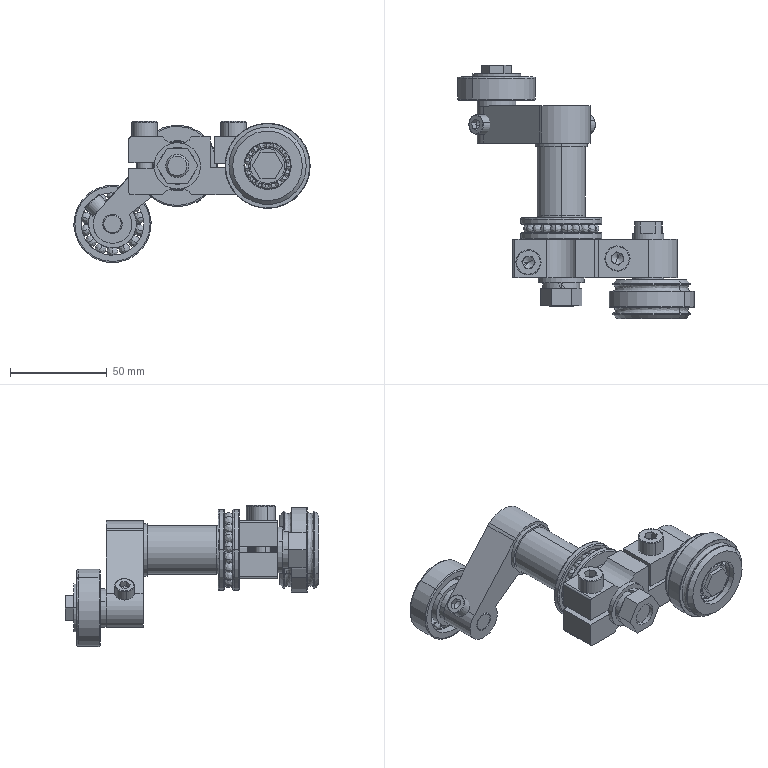Part | SolidWorks | 23 solids | 1284 faces | box 122.175 x 130.9 x 73.017 mm | volume 147727 mm3 | cylinder 483 | spline 403 | plane 362 | cone 36 | commonest cylinder face diameters 0.75 x215 16.285 x95 8 x8 10 x8 19.333 x8 23.667 x8